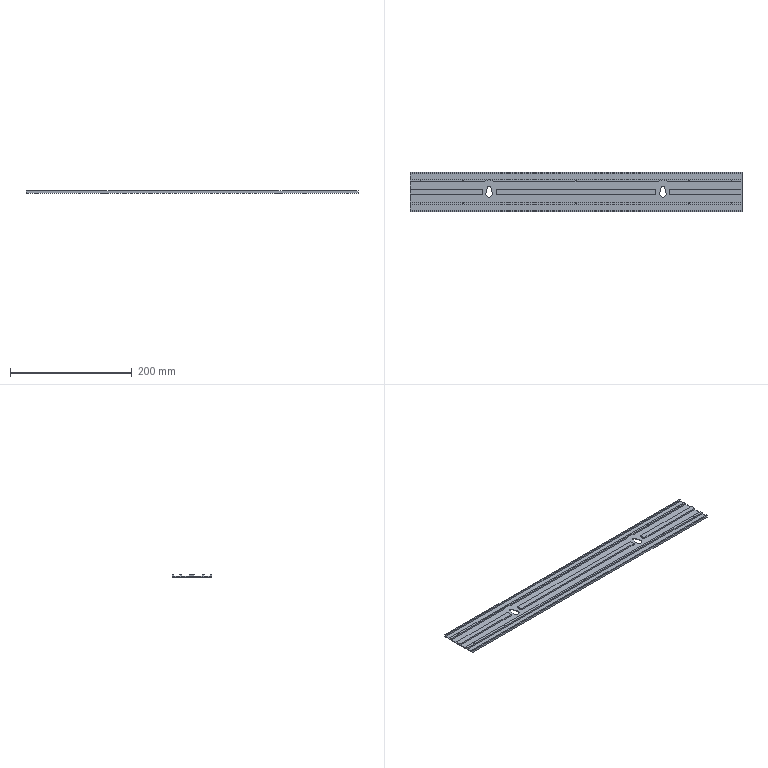Part | NX | features solid 2 | 1 solid | 89 faces | box 544.5 x 64 x 3.5 mm | volume 58637 mm3 | plane 38 | cylinder 31 | cone 20 | commonest cylinder face diameters 1.25 x20 23 x6 5.25 x2 10.5 x2 3.742 x1